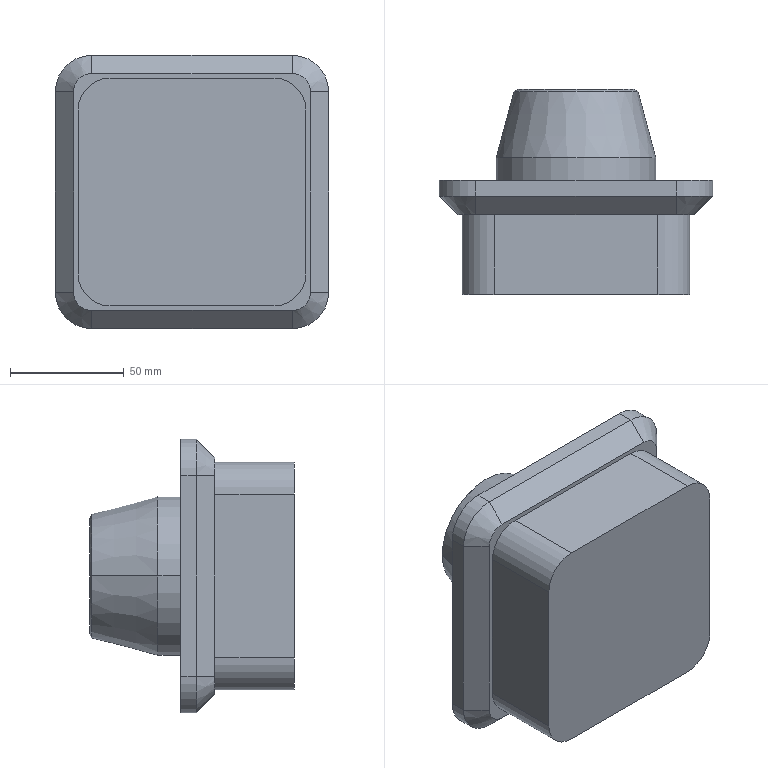Part | SolidWorks | features Chamfer 2, ICE 2, Revolution 1 | 1 solid | 34 faces | box 120 x 90 x 120 mm | volume 672208 mm3 | plane 16 | cylinder 10 | cone 8 | commonest cylinder face diameters 28 x4 32 x4 70 x2
STEP:
#1=CARTESIAN_POINT('',(-25.547,40.,0.));
#2=VERTEX_POINT('',#1);
#3=CARTESIAN_POINT('',(25.547,40.,0.));
#4=VERTEX_POINT('',#3);
#5=CARTESIAN_POINT('',(0.,40.,0.));
#6=DIRECTION('',(0.,1.,0.));
#7=DIRECTION('',(1.,0.,0.));
#8=AXIS2_PLACEMENT_3D('',#5,#6,#7);
#9=CIRCLE('',#8,25.547);
#10=EDGE_CURVE('',#2,#4,#9,.T.);
#11=ORIENTED_EDGE('',*,*,#10,.F.);
#12=CARTESIAN_POINT('',(-27.22,39.034,0.));
#13=VERTEX_POINT('',#12);
#14=CARTESIAN_POINT('',(-25.547,40.,0.));
#15=DIRECTION('',(-0.866,-0.5,0.));
#16=VECTOR('',#15,1000.);
#17=LINE('',#14,#16);
#18=EDGE_CURVE('',#2,#13,#17,.T.);
#19=ORIENTED_EDGE('',*,*,#18,.T.);
#20=CARTESIAN_POINT('',(27.22,39.034,0.));
#21=VERTEX_POINT('',#20);
#22=CARTESIAN_POINT('',(0.,39.034,0.));
#23=DIRECTION('',(0.,-1.,0.));
#24=DIRECTION('',(-1.,0.,0.));
#25=AXIS2_PLACEMENT_3D('',#22,#23,#24);
#26=CIRCLE('',#25,27.22);
#27=EDGE_CURVE('',#21,#13,#26,.T.);
#28=ORIENTED_EDGE('',*,*,#27,.F.);
#29=CARTESIAN_POINT('',(25.547,40.,0.));
#30=DIRECTION('',(0.866,-0.5,0.));
#31=VECTOR('',#30,1000.);
#32=LINE('',#29,#31);
#33=EDGE_CURVE('',#4,#21,#32,.T.);
#34=ORIENTED_EDGE('',*,*,#33,.F.);
#35=EDGE_LOOP('',(#11,#19,#28,#34));
#36=FACE_OUTER_BOUND('',#35,.T.);
#37=CARTESIAN_POINT('',(0.,40.,0.));
#38=DIRECTION('',(0.,-1.,0.));
#39=DIRECTION('',(1.,0.,0.));
#40=AXIS2_PLACEMENT_3D('',#37,#38,#39);
#41=CONICAL_SURFACE('',#40,25.547,1.047);
#42=ADVANCED_FACE('',(#36),#41,.T.);
#43=ORIENTED_EDGE('',*,*,#27,.T.);
#44=CARTESIAN_POINT('',(-35.,10.,0.));
#45=VERTEX_POINT('',#44);
#46=CARTESIAN_POINT('',(-35.,10.,0.));
#47=DIRECTION('',(-0.2588,-0.9659,0.));
#48=VECTOR('',#47,1000.);
#49=LINE('',#46,#48);
#50=EDGE_CURVE('',#13,#45,#49,.T.);
#51=ORIENTED_EDGE('',*,*,#50,.T.);
#52=CARTESIAN_POINT('',(35.,10.,0.));
#53=VERTEX_POINT('',#52);
#54=CARTESIAN_POINT('',(0.,10.,0.));
#55=DIRECTION('',(0.,1.,0.));
#56=DIRECTION('',(-1.,0.,0.));
#57=AXIS2_PLACEMENT_3D('',#54,#55,#56);
#58=CIRCLE('',#57,35.);
#59=EDGE_CURVE('',#45,#53,#58,.T.);
#60=ORIENTED_EDGE('',*,*,#59,.T.);
#61=CARTESIAN_POINT('',(35.,10.,0.));
#62=DIRECTION('',(0.2588,-0.9659,0.));
#63=VECTOR('',#62,1000.);
#64=LINE('',#61,#63);
#65=EDGE_CURVE('',#21,#53,#64,.T.);
#66=ORIENTED_EDGE('',*,*,#65,.F.);
#67=EDGE_LOOP('',(#43,#51,#60,#66));
#68=FACE_OUTER_BOUND('',#67,.T.);
#69=CARTESIAN_POINT('',(0.,10.,0.));
#70=DIRECTION('',(0.,-1.,0.));
#71=DIRECTION('',(1.,0.,0.));
#72=AXIS2_PLACEMENT_3D('',#69,#70,#71);
#73=CONICAL_SURFACE('',#72,35.,0.2618);
#74=ADVANCED_FACE('',(#68),#73,.T.);
#75=CARTESIAN_POINT('',(-35.,0.,0.));
#76=VERTEX_POINT('',#75);
#77=CARTESIAN_POINT('',(35.,0.,0.));
#78=VERTEX_POINT('',#77);
#79=CARTESIAN_POINT('',(0.,0.,0.));
#80=DIRECTION('',(0.,1.,0.));
#81=DIRECTION('',(-1.,0.,0.));
#82=AXIS2_PLACEMENT_3D('',#79,#80,#81);
#83=CIRCLE('',#82,35.);
#84=EDGE_CURVE('',#76,#78,#83,.T.);
#85=ORIENTED_EDGE('',*,*,#84,.T.);
#86=CARTESIAN_POINT('',(35.,40.,0.));
#87=DIRECTION('',(0.,1.,0.));
#88=VECTOR('',#87,1000.);
#89=LINE('',#86,#88);
#90=EDGE_CURVE('',#78,#53,#89,.T.);
#91=ORIENTED_EDGE('',*,*,#90,.T.);
#92=ORIENTED_EDGE('',*,*,#59,.F.);
#93=CARTESIAN_POINT('',(-35.,40.,0.));
#94=DIRECTION('',(0.,1.,0.));
#95=VECTOR('',#94,1000.);
#96=LINE('',#93,#95);
#97=EDGE_CURVE('',#76,#45,#96,.T.);
#98=ORIENTED_EDGE('',*,*,#97,.F.);
#99=EDGE_LOOP('',(#85,#91,#92,#98));
#100=FACE_OUTER_BOUND('',#99,.T.);
#101=CARTESIAN_POINT('',(0.,40.,0.));
#102=DIRECTION('',(0.,1.,0.));
#103=DIRECTION('',(-1.,0.,0.));
#104=AXIS2_PLACEMENT_3D('',#101,#102,#103);
#105=CYLINDRICAL_SURFACE('',#104,35.);
#106=ADVANCED_FACE('',(#100),#105,.T.);
#107=CARTESIAN_POINT('',(-52.,-15.,44.));
#108=VERTEX_POINT('',#107);
#109=CARTESIAN_POINT('',(-52.,-15.,-44.));
#110=VERTEX_POINT('',#109);
#111=CARTESIAN_POINT('',(-52.,-15.,-44.));
#112=DIRECTION('',(0.,0.,-1.));
#113=VECTOR('',#112,1000.);
#114=LINE('',#111,#113);
#115=EDGE_CURVE('',#108,#110,#114,.T.);
#116=ORIENTED_EDGE('',*,*,#115,.T.);
#117=CARTESIAN_POINT('',(-44.,-15.,-52.));
#118=VERTEX_POINT('',#117);
#119=CARTESIAN_POINT('',(-44.,-15.,-44.));
#120=DIRECTION('',(0.,-1.,0.));
#121=DIRECTION('',(-1.,0.,0.));
#122=AXIS2_PLACEMENT_3D('',#119,#120,#121);
#123=CIRCLE('',#122,8.);
#124=EDGE_CURVE('',#110,#118,#123,.T.);
#125=ORIENTED_EDGE('',*,*,#124,.T.);
#126=CARTESIAN_POINT('',(44.,-15.,-52.));
#127=VERTEX_POINT('',#126);
#128=CARTESIAN_POINT('',(-44.,-15.,-52.));
#129=DIRECTION('',(1.,0.,0.));
#130=VECTOR('',#129,1000.);
#131=LINE('',#128,#130);
#132=EDGE_CURVE('',#118,#127,#131,.T.);
#133=ORIENTED_EDGE('',*,*,#132,.T.);
#134=CARTESIAN_POINT('',(52.,-15.,-44.));
#135=VERTEX_POINT('',#134);
#136=CARTESIAN_POINT('',(44.,-15.,-44.));
#137=DIRECTION('',(0.,-1.,0.));
#138=DIRECTION('',(-1.,0.,0.));
#139=AXIS2_PLACEMENT_3D('',#136,#137,#138);
#140=CIRCLE('',#139,8.);
#141=EDGE_CURVE('',#127,#135,#140,.T.);
#142=ORIENTED_EDGE('',*,*,#141,.T.);
#143=CARTESIAN_POINT('',(52.,-15.,44.));
#144=VERTEX_POINT('',#143);
#145=CARTESIAN_POINT('',(52.,-15.,-44.));
#146=DIRECTION('',(0.,0.,1.));
#147=VECTOR('',#146,1000.);
#148=LINE('',#145,#147);
#149=EDGE_CURVE('',#135,#144,#148,.T.);
#150=ORIENTED_EDGE('',*,*,#149,.T.);
#151=CARTESIAN_POINT('',(44.,-15.,52.));
#152=VERTEX_POINT('',#151);
#153=CARTESIAN_POINT('',(44.,-15.,44.));
#154=DIRECTION('',(0.,-1.,0.));
#155=DIRECTION('',(-1.,0.,0.));
#156=AXIS2_PLACEMENT_3D('',#153,#154,#155);
#157=CIRCLE('',#156,8.);
#158=EDGE_CURVE('',#144,#152,#157,.T.);
#159=ORIENTED_EDGE('',*,*,#158,.T.);
#160=CARTESIAN_POINT('',(-44.,-15.,52.));
#161=VERTEX_POINT('',#160);
#162=CARTESIAN_POINT('',(-44.,-15.,52.));
#163=DIRECTION('',(-1.,0.,0.));
#164=VECTOR('',#163,1000.);
#165=LINE('',#162,#164);
#166=EDGE_CURVE('',#152,#161,#165,.T.);
#167=ORIENTED_EDGE('',*,*,#166,.T.);
#168=CARTESIAN_POINT('',(-44.,-15.,44.));
#169=DIRECTION('',(0.,-1.,0.));
#170=DIRECTION('',(-1.,0.,0.));
#171=AXIS2_PLACEMENT_3D('',#168,#169,#170);
#172=CIRCLE('',#171,8.);
#173=EDGE_CURVE('',#161,#108,#172,.T.);
#174=ORIENTED_EDGE('',*,*,#173,.T.);
#175=EDGE_LOOP('',(#116,#125,#133,#142,#150,#159,#167,#174));
#176=FACE_OUTER_BOUND('',#175,.T.);
#177=CARTESIAN_POINT('',(-50.,-15.,-36.));
#178=VERTEX_POINT('',#177);
#179=CARTESIAN_POINT('',(-36.,-15.,-50.));
#180=VERTEX_POINT('',#179);
#181=CARTESIAN_POINT('',(-36.,-15.,-36.));
#182=DIRECTION('',(0.,-1.,0.));
#183=DIRECTION('',(-1.,0.,0.));
#184=AXIS2_PLACEMENT_3D('',#181,#182,#183);
#185=CIRCLE('',#184,14.);
#186=EDGE_CURVE('',#178,#180,#185,.T.);
#187=ORIENTED_EDGE('',*,*,#186,.F.);
#188=CARTESIAN_POINT('',(-50.,-15.,36.));
#189=VERTEX_POINT('',#188);
#190=CARTESIAN_POINT('',(-50.,-15.,-36.));
#191=DIRECTION('',(0.,0.,-1.));
#192=VECTOR('',#191,1000.);
#193=LINE('',#190,#192);
#194=EDGE_CURVE('',#189,#178,#193,.T.);
#195=ORIENTED_EDGE('',*,*,#194,.F.);
#196=CARTESIAN_POINT('',(-36.,-15.,50.));
#197=VERTEX_POINT('',#196);
#198=CARTESIAN_POINT('',(-36.,-15.,36.));
#199=DIRECTION('',(0.,-1.,0.));
#200=DIRECTION('',(1.,0.,0.));
#201=AXIS2_PLACEMENT_3D('',#198,#199,#200);
#202=CIRCLE('',#201,14.);
#203=EDGE_CURVE('',#197,#189,#202,.T.);
#204=ORIENTED_EDGE('',*,*,#203,.F.);
#205=CARTESIAN_POINT('',(36.,-15.,50.));
#206=VERTEX_POINT('',#205);
#207=CARTESIAN_POINT('',(36.,-15.,50.));
#208=DIRECTION('',(-1.,0.,0.));
#209=VECTOR('',#208,1000.);
#210=LINE('',#207,#209);
#211=EDGE_CURVE('',#206,#197,#210,.T.);
#212=ORIENTED_EDGE('',*,*,#211,.F.);
#213=CARTESIAN_POINT('',(50.,-15.,36.));
#214=VERTEX_POINT('',#213);
#215=CARTESIAN_POINT('',(36.,-15.,36.));
#216=DIRECTION('',(0.,-1.,0.));
#217=DIRECTION('',(1.,0.,0.));
#218=AXIS2_PLACEMENT_3D('',#215,#216,#217);
#219=CIRCLE('',#218,14.);
#220=EDGE_CURVE('',#214,#206,#219,.T.);
#221=ORIENTED_EDGE('',*,*,#220,.F.);
#222=CARTESIAN_POINT('',(50.,-15.,-36.));
#223=VERTEX_POINT('',#222);
#224=CARTESIAN_POINT('',(50.,-15.,-36.));
#225=DIRECTION('',(0.,0.,1.));
#226=VECTOR('',#225,1000.);
#227=LINE('',#224,#226);
#228=EDGE_CURVE('',#223,#214,#227,.T.);
#229=ORIENTED_EDGE('',*,*,#228,.F.);
#230=CARTESIAN_POINT('',(36.,-15.,-50.));
#231=VERTEX_POINT('',#230);
#232=CARTESIAN_POINT('',(36.,-15.,-36.));
#233=DIRECTION('',(0.,-1.,0.));
#234=DIRECTION('',(1.,0.,0.));
#235=AXIS2_PLACEMENT_3D('',#232,#233,#234);
#236=CIRCLE('',#235,14.);
#237=EDGE_CURVE('',#231,#223,#236,.T.);
#238=ORIENTED_EDGE('',*,*,#237,.F.);
#239=CARTESIAN_POINT('',(36.,-15.,-50.));
#240=DIRECTION('',(1.,0.,0.));
#241=VECTOR('',#240,1000.);
#242=LINE('',#239,#241);
#243=EDGE_CURVE('',#180,#231,#242,.T.);
#244=ORIENTED_EDGE('',*,*,#243,.F.);
#245=EDGE_LOOP('',(#187,#195,#204,#212,#221,#229,#238,#244));
#246=FACE_BOUND('',#245,.T.);
#247=CARTESIAN_POINT('',(-44.,-15.,-44.));
#248=DIRECTION('',(0.,1.,0.));
#249=DIRECTION('',(-1.,0.,0.));
#250=AXIS2_PLACEMENT_3D('',#247,#248,#249);
#251=PLANE('',#250);
#252=ADVANCED_FACE('',(#176,#246),#251,.F.);
#253=ORIENTED_EDGE('',*,*,#90,.F.);
#254=CARTESIAN_POINT('',(0.,0.,0.));
#255=DIRECTION('',(0.,1.,0.));
#256=DIRECTION('',(-1.,0.,0.));
#257=AXIS2_PLACEMENT_3D('',#254,#255,#256);
#258=CIRCLE('',#257,35.);
#259=EDGE_CURVE('',#78,#76,#258,.T.);
#260=ORIENTED_EDGE('',*,*,#259,.T.);
#261=ORIENTED_EDGE('',*,*,#97,.T.);
#262=CARTESIAN_POINT('',(0.,10.,0.));
#263=DIRECTION('',(0.,1.,0.));
#264=DIRECTION('',(-1.,0.,0.));
#265=AXIS2_PLACEMENT_3D('',#262,#263,#264);
#266=CIRCLE('',#265,35.);
#267=EDGE_CURVE('',#53,#45,#266,.T.);
#268=ORIENTED_EDGE('',*,*,#267,.F.);
#269=EDGE_LOOP('',(#253,#260,#261,#268));
#270=FACE_OUTER_BOUND('',#269,.T.);
#271=CARTESIAN_POINT('',(0.,40.,0.));
#272=DIRECTION('',(0.,1.,0.));
#273=DIRECTION('',(-1.,0.,0.));
#274=AXIS2_PLACEMENT_3D('',#271,#272,#273);
#275=CYLINDRICAL_SURFACE('',#274,35.);
#276=ADVANCED_FACE('',(#270),#275,.T.);
#277=ORIENTED_EDGE('',*,*,#50,.F.);
#278=CARTESIAN_POINT('',(0.,39.034,0.));
#279=DIRECTION('',(0.,-1.,0.));
#280=DIRECTION('',(-1.,0.,0.));
#281=AXIS2_PLACEMENT_3D('',#278,#279,#280);
#282=CIRCLE('',#281,27.22);
#283=EDGE_CURVE('',#13,#21,#282,.T.);
#284=ORIENTED_EDGE('',*,*,#283,.T.);
#285=ORIENTED_EDGE('',*,*,#65,.T.);
#286=ORIENTED_EDGE('',*,*,#267,.T.);
#287=EDGE_LOOP('',(#277,#284,#285,#286));
#288=FACE_OUTER_BOUND('',#287,.T.);
#289=CARTESIAN_POINT('',(0.,10.,0.));
#290=DIRECTION('',(0.,-1.,0.));
#291=DIRECTION('',(1.,0.,0.));
#292=AXIS2_PLACEMENT_3D('',#289,#290,#291);
#293=CONICAL_SURFACE('',#292,35.,0.2618);
#294=ADVANCED_FACE('',(#288),#293,.T.);
#295=CARTESIAN_POINT('',(0.,40.,0.));
#296=DIRECTION('',(0.,1.,0.));
#297=DIRECTION('',(1.,0.,0.));
#298=AXIS2_PLACEMENT_3D('',#295,#296,#297);
#299=CIRCLE('',#298,25.547);
#300=EDGE_CURVE('',#4,#2,#299,.T.);
#301=ORIENTED_EDGE('',*,*,#300,.T.);
#302=ORIENTED_EDGE('',*,*,#10,.T.);
#303=EDGE_LOOP('',(#301,#302));
#304=FACE_OUTER_BOUND('',#303,.T.);
#305=CARTESIAN_POINT('',(26.962,40.,0.));
#306=DIRECTION('',(0.,-1.,0.));
#307=DIRECTION('',(1.,0.,0.));
#308=AXIS2_PLACEMENT_3D('',#305,#306,#307);
#309=PLANE('',#308);
#310=ADVANCED_FACE('',(#304),#309,.F.);
#311=ORIENTED_EDGE('',*,*,#18,.F.);
#312=ORIENTED_EDGE('',*,*,#300,.F.);
#313=ORIENTED_EDGE('',*,*,#33,.T.);
#314=ORIENTED_EDGE('',*,*,#283,.F.);
#315=EDGE_LOOP('',(#311,#312,#313,#314));
#316=FACE_OUTER_BOUND('',#315,.T.);
#317=CARTESIAN_POINT('',(0.,40.,0.));
#318=DIRECTION('',(0.,-1.,0.));
#319=DIRECTION('',(1.,0.,0.));
#320=AXIS2_PLACEMENT_3D('',#317,#318,#319);
#321=CONICAL_SURFACE('',#320,25.547,1.047);
#322=ADVANCED_FACE('',(#316),#321,.T.);
#323=CARTESIAN_POINT('',(-44.,-7.,-60.));
#324=VERTEX_POINT('',#323);
#325=CARTESIAN_POINT('',(-44.,0.,-60.));
#326=VERTEX_POINT('',#325);
#327=CARTESIAN_POINT('',(-44.,-15.,-60.));
#328=DIRECTION('',(0.,1.,0.));
#329=VECTOR('',#328,1000.);
#330=LINE('',#327,#329);
#331=EDGE_CURVE('',#324,#326,#330,.T.);
#332=ORIENTED_EDGE('',*,*,#331,.F.);
#333=CARTESIAN_POINT('',(-60.,-7.,-44.));
#334=VERTEX_POINT('',#333);
#335=CARTESIAN_POINT('',(-44.,-7.,-44.));
#336=DIRECTION('',(0.,1.,0.));
#337=DIRECTION('',(0.,0.,1.));
#338=AXIS2_PLACEMENT_3D('',#335,#336,#337);
#339=CIRCLE('',#338,16.);
#340=EDGE_CURVE('',#324,#334,#339,.T.);
#341=ORIENTED_EDGE('',*,*,#340,.T.);
#342=CARTESIAN_POINT('',(-60.,0.,-44.));
#343=VERTEX_POINT('',#342);
#344=CARTESIAN_POINT('',(-60.,-15.,-44.));
#345=DIRECTION('',(0.,1.,0.));
#346=VECTOR('',#345,1000.);
#347=LINE('',#344,#346);
#348=EDGE_CURVE('',#334,#343,#347,.T.);
#349=ORIENTED_EDGE('',*,*,#348,.T.);
#350=CARTESIAN_POINT('',(-44.,0.,-44.));
#351=DIRECTION('',(0.,-1.,0.));
#352=DIRECTION('',(-1.,0.,0.));
#353=AXIS2_PLACEMENT_3D('',#350,#351,#352);
#354=CIRCLE('',#353,16.);
#355=EDGE_CURVE('',#343,#326,#354,.T.);
#356=ORIENTED_EDGE('',*,*,#355,.T.);
#357=EDGE_LOOP('',(#332,#341,#349,#356));
#358=FACE_OUTER_BOUND('',#357,.T.);
#359=CARTESIAN_POINT('',(-44.,-15.,-44.));
#360=DIRECTION('',(0.,1.,0.));
#361=DIRECTION('',(-1.,0.,0.));
#362=AXIS2_PLACEMENT_3D('',#359,#360,#361);
#363=CYLINDRICAL_SURFACE('',#362,16.);
#364=ADVANCED_FACE('',(#358),#363,.T.);
#365=CARTESIAN_POINT('',(44.,-7.,-60.));
#366=VERTEX_POINT('',#365);
#367=CARTESIAN_POINT('',(44.,0.,-60.));
#368=VERTEX_POINT('',#367);
#369=CARTESIAN_POINT('',(44.,-15.,-60.));
#370=DIRECTION('',(0.,1.,0.));
#371=VECTOR('',#370,1000.);
#372=LINE('',#369,#371);
#373=EDGE_CURVE('',#366,#368,#372,.T.);
#374=ORIENTED_EDGE('',*,*,#373,.F.);
#375=CARTESIAN_POINT('',(44.,-7.,-60.));
#376=DIRECTION('',(-1.,0.,0.));
#377=VECTOR('',#376,1000.);
#378=LINE('',#375,#377);
#379=EDGE_CURVE('',#366,#324,#378,.T.);
#380=ORIENTED_EDGE('',*,*,#379,.T.);
#381=ORIENTED_EDGE('',*,*,#331,.T.);
#382=CARTESIAN_POINT('',(44.,0.,-60.));
#383=DIRECTION('',(1.,0.,0.));
#384=VECTOR('',#383,1000.);
#385=LINE('',#382,#384);
#386=EDGE_CURVE('',#326,#368,#385,.T.);
#387=ORIENTED_EDGE('',*,*,#386,.T.);
#388=EDGE_LOOP('',(#374,#380,#381,#387));
#389=FACE_OUTER_BOUND('',#388,.T.);
#390=CARTESIAN_POINT('',(44.,-15.,-60.));
#391=DIRECTION('',(0.,0.,1.));
#392=DIRECTION('',(1.,0.,0.));
#393=AXIS2_PLACEMENT_3D('',#390,#391,#392);
#394=PLANE('',#393);
#395=ADVANCED_FACE('',(#389),#394,.F.);
#396=CARTESIAN_POINT('',(60.,-7.,-44.));
#397=VERTEX_POINT('',#396);
#398=CARTESIAN_POINT('',(60.,0.,-44.));
#399=VERTEX_POINT('',#398);
#400=CARTESIAN_POINT('',(60.,-15.,-44.));
#401=DIRECTION('',(0.,1.,0.));
#402=VECTOR('',#401,1000.);
#403=LINE('',#400,#402);
#404=EDGE_CURVE('',#397,#399,#403,.T.);
#405=ORIENTED_EDGE('',*,*,#404,.F.);
#406=CARTESIAN_POINT('',(44.,-7.,-44.));
#407=DIRECTION('',(0.,1.,0.));
#408=DIRECTION('',(0.,0.,1.));
#409=AXIS2_PLACEMENT_3D('',#406,#407,#408);
#410=CIRCLE('',#409,16.);
#411=EDGE_CURVE('',#397,#366,#410,.T.);
#412=ORIENTED_EDGE('',*,*,#411,.T.);
#413=ORIENTED_EDGE('',*,*,#373,.T.);
#414=CARTESIAN_POINT('',(44.,0.,-44.));
#415=DIRECTION('',(0.,-1.,0.));
#416=DIRECTION('',(1.,0.,0.));
#417=AXIS2_PLACEMENT_3D('',#414,#415,#416);
#418=CIRCLE('',#417,16.);
#419=EDGE_CURVE('',#368,#399,#418,.T.);
#420=ORIENTED_EDGE('',*,*,#419,.T.);
#421=EDGE_LOOP('',(#405,#412,#413,#420));
#422=FACE_OUTER_BOUND('',#421,.T.);
#423=CARTESIAN_POINT('',(44.,-15.,-44.));
#424=DIRECTION('',(0.,1.,0.));
#425=DIRECTION('',(-1.,0.,0.));
#426=AXIS2_PLACEMENT_3D('',#423,#424,#425);
#427=CYLINDRICAL_SURFACE('',#426,16.);
#428=ADVANCED_FACE('',(#422),#427,.T.);
#429=CARTESIAN_POINT('',(60.,-7.,44.));
#430=VERTEX_POINT('',#429);
#431=CARTESIAN_POINT('',(60.,0.,44.));
#432=VERTEX_POINT('',#431);
#433=CARTESIAN_POINT('',(60.,-15.,44.));
#434=DIRECTION('',(0.,1.,0.));
#435=VECTOR('',#434,1000.);
#436=LINE('',#433,#435);
#437=EDGE_CURVE('',#430,#432,#436,.T.);
#438=ORIENTED_EDGE('',*,*,#437,.F.);
#439=CARTESIAN_POINT('',(60.,-7.,-44.));
#440=DIRECTION('',(0.,0.,-1.));
#441=VECTOR('',#440,1000.);
#442=LINE('',#439,#441);
#443=EDGE_CURVE('',#430,#397,#442,.T.);
#444=ORIENTED_EDGE('',*,*,#443,.T.);
#445=ORIENTED_EDGE('',*,*,#404,.T.);
#446=CARTESIAN_POINT('',(60.,0.,-44.));
#447=DIRECTION('',(0.,0.,1.));
#448=VECTOR('',#447,1000.);
#449=LINE('',#446,#448);
#450=EDGE_CURVE('',#399,#432,#449,.T.);
#451=ORIENTED_EDGE('',*,*,#450,.T.);
#452=EDGE_LOOP('',(#438,#444,#445,#451));
#453=FACE_OUTER_BOUND('',#452,.T.);
#454=CARTESIAN_POINT('',(60.,-15.,-44.));
#455=DIRECTION('',(-1.,0.,0.));
#456=DIRECTION('',(0.,-1.,0.));
#457=AXIS2_PLACEMENT_3D('',#454,#455,#456);
#458=PLANE('',#457);
#459=ADVANCED_FACE('',(#453),#458,.F.);
#460=CARTESIAN_POINT('',(44.,-7.,60.));
#461=VERTEX_POINT('',#460);
#462=CARTESIAN_POINT('',(44.,0.,60.));
#463=VERTEX_POINT('',#462);
#464=CARTESIAN_POINT('',(44.,-15.,60.));
#465=DIRECTION('',(0.,1.,0.));
#466=VECTOR('',#465,1000.);
#467=LINE('',#464,#466);
#468=EDGE_CURVE('',#461,#463,#467,.T.);
#469=ORIENTED_EDGE('',*,*,#468,.F.);
#470=CARTESIAN_POINT('',(44.,-7.,44.));
#471=DIRECTION('',(0.,1.,0.));
#472=DIRECTION('',(0.,0.,1.));
#473=AXIS2_PLACEMENT_3D('',#470,#471,#472);
#474=CIRCLE('',#473,16.);
#475=EDGE_CURVE('',#461,#430,#474,.T.);
#476=ORIENTED_EDGE('',*,*,#475,.T.);
#477=ORIENTED_EDGE('',*,*,#437,.T.);
#478=CARTESIAN_POINT('',(44.,0.,44.));
#479=DIRECTION('',(0.,-1.,0.));
#480=DIRECTION('',(1.,0.,0.));
#481=AXIS2_PLACEMENT_3D('',#478,#479,#480);
#482=CIRCLE('',#481,16.);
#483=EDGE_CURVE('',#432,#463,#482,.T.);
#484=ORIENTED_EDGE('',*,*,#483,.T.);
#485=EDGE_LOOP('',(#469,#476,#477,#484));
#486=FACE_OUTER_BOUND('',#485,.T.);
#487=CARTESIAN_POINT('',(44.,-15.,44.));
#488=DIRECTION('',(0.,1.,0.));
#489=DIRECTION('',(-1.,0.,0.));
#490=AXIS2_PLACEMENT_3D('',#487,#488,#489);
#491=CYLINDRICAL_SURFACE('',#490,16.);
#492=ADVANCED_FACE('',(#486),#491,.T.);
#493=CARTESIAN_POINT('',(-44.,-7.,60.));
#494=VERTEX_POINT('',#493);
#495=CARTESIAN_POINT('',(-44.,0.,60.));
#496=VERTEX_POINT('',#495);
#497=CARTESIAN_POINT('',(-44.,-15.,60.));
#498=DIRECTION('',(0.,1.,0.));
#499=VECTOR('',#498,1000.);
#500=LINE('',#497,#499);
#501=EDGE_CURVE('',#494,#496,#500,.T.);
#502=ORIENTED_EDGE('',*,*,#501,.F.);
#503=CARTESIAN_POINT('',(44.,-7.,60.));
#504=DIRECTION('',(1.,0.,0.));
#505=VECTOR('',#504,1000.);
#506=LINE('',#503,#505);
#507=EDGE_CURVE('',#494,#461,#506,.T.);
#508=ORIENTED_EDGE('',*,*,#507,.T.);
#509=ORIENTED_EDGE('',*,*,#468,.T.);
#510=CARTESIAN_POINT('',(44.,0.,60.));
#511=DIRECTION('',(-1.,0.,0.));
#512=VECTOR('',#511,1000.);
#513=LINE('',#510,#512);
#514=EDGE_CURVE('',#463,#496,#513,.T.);
#515=ORIENTED_EDGE('',*,*,#514,.T.);
#516=EDGE_LOOP('',(#502,#508,#509,#515));
#517=FACE_OUTER_BOUND('',#516,.T.);
#518=CARTESIAN_POINT('',(44.,-15.,60.));
#519=DIRECTION('',(0.,0.,-1.));
#520=DIRECTION('',(-1.,0.,0.));
#521=AXIS2_PLACEMENT_3D('',#518,#519,#520);
#522=PLANE('',#521);
#523=ADVANCED_FACE('',(#517),#522,.F.);
#524=CARTESIAN_POINT('',(-60.,-7.,44.));
#525=VERTEX_POINT('',#524);
#526=CARTESIAN_POINT('',(-60.,0.,44.));
#527=VERTEX_POINT('',#526);
#528=CARTESIAN_POINT('',(-60.,-15.,44.));
#529=DIRECTION('',(0.,1.,0.));
#530=VECTOR('',#529,1000.);
#531=LINE('',#528,#530);
#532=EDGE_CURVE('',#525,#527,#531,.T.);
#533=ORIENTED_EDGE('',*,*,#532,.F.);
#534=CARTESIAN_POINT('',(-44.,-7.,44.));
#535=DIRECTION('',(0.,1.,0.));
#536=DIRECTION('',(0.,0.,1.));
#537=AXIS2_PLACEMENT_3D('',#534,#535,#536);
#538=CIRCLE('',#537,16.);
#539=EDGE_CURVE('',#525,#494,#538,.T.);
#540=ORIENTED_EDGE('',*,*,#539,.T.);
#541=ORIENTED_EDGE('',*,*,#501,.T.);
#542=CARTESIAN_POINT('',(-44.,0.,44.));
#543=DIRECTION('',(0.,-1.,0.));
#544=DIRECTION('',(1.,0.,0.));
#545=AXIS2_PLACEMENT_3D('',#542,#543,#544);
#546=CIRCLE('',#545,16.);
#547=EDGE_CURVE('',#496,#527,#546,.T.);
#548=ORIENTED_EDGE('',*,*,#547,.T.);
#549=EDGE_LOOP('',(#533,#540,#541,#548));
#550=FACE_OUTER_BOUND('',#549,.T.);
#551=CARTESIAN_POINT('',(-44.,-15.,44.));
#552=DIRECTION('',(0.,1.,0.));
#553=DIRECTION('',(-1.,0.,0.));
#554=AXIS2_PLACEMENT_3D('',#551,#552,#553);
#555=CYLINDRICAL_SURFACE('',#554,16.);
#556=ADVANCED_FACE('',(#550),#555,.T.);
#557=ORIENTED_EDGE('',*,*,#348,.F.);
#558=CARTESIAN_POINT('',(-60.,-7.,-44.));
#559=DIRECTION('',(0.,0.,1.));
#560=VECTOR('',#559,1000.);
#561=LINE('',#558,#560);
#562=EDGE_CURVE('',#334,#525,#561,.T.);
#563=ORIENTED_EDGE('',*,*,#562,.T.);
#564=ORIENTED_EDGE('',*,*,#532,.T.);
#565=CARTESIAN_POINT('',(-60.,0.,-44.));
#566=DIRECTION('',(0.,0.,-1.));
#567=VECTOR('',#566,1000.);
#568=LINE('',#565,#567);
#569=EDGE_CURVE('',#527,#343,#568,.T.);
#570=ORIENTED_EDGE('',*,*,#569,.T.);
#571=EDGE_LOOP('',(#557,#563,#564,#570));
#572=FACE_OUTER_BOUND('',#571,.T.);
#573=CARTESIAN_POINT('',(-60.,-15.,-44.));
#574=DIRECTION('',(1.,0.,0.));
#575=DIRECTION('',(0.,0.,-1.));
#576=AXIS2_PLACEMENT_3D('',#573,#574,#575);
#577=PLANE('',#576);
#578=ADVANCED_FACE('',(#572),#577,.F.);
#579=ORIENTED_EDGE('',*,*,#84,.F.);
#580=ORIENTED_EDGE('',*,*,#259,.F.);
#581=EDGE_LOOP('',(#579,#580));
#582=FACE_BOUND('',#581,.T.);
#583=ORIENTED_EDGE('',*,*,#355,.F.);
#584=ORIENTED_EDGE('',*,*,#569,.F.);
#585=ORIENTED_EDGE('',*,*,#547,.F.);
#586=ORIENTED_EDGE('',*,*,#514,.F.);
#587=ORIENTED_EDGE('',*,*,#483,.F.);
#588=ORIENTED_EDGE('',*,*,#450,.F.);
#589=ORIENTED_EDGE('',*,*,#419,.F.);
#590=ORIENTED_EDGE('',*,*,#386,.F.);
#591=EDGE_LOOP('',(#583,#584,#585,#586,#587,#588,#589,#590));
#592=FACE_OUTER_BOUND('',#591,.T.);
#593=CARTESIAN_POINT('',(-44.,0.,-44.));
#594=DIRECTION('',(0.,1.,0.));
#595=DIRECTION('',(-1.,0.,0.));
#596=AXIS2_PLACEMENT_3D('',#593,#594,#595);
#597=PLANE('',#596);
#598=ADVANCED_FACE('',(#582,#592),#597,.T.);
#599=ORIENTED_EDGE('',*,*,#186,.T.);
#600=CARTESIAN_POINT('',(-36.,-50.,-50.));
#601=VERTEX_POINT('',#600);
#602=CARTESIAN_POINT('',(-36.,-50.,-50.));
#603=DIRECTION('',(0.,1.,0.));
#604=VECTOR('',#603,1000.);
#605=LINE('',#602,#604);
#606=EDGE_CURVE('',#601,#180,#605,.T.);
#607=ORIENTED_EDGE('',*,*,#606,.F.);
#608=CARTESIAN_POINT('',(-50.,-50.,-36.));
#609=VERTEX_POINT('',#608);
#610=CARTESIAN_POINT('',(-36.,-50.,-36.));
#611=DIRECTION('',(0.,-1.,0.));
#612=DIRECTION('',(-1.,0.,0.));
#613=AXIS2_PLACEMENT_3D('',#610,#611,#612);
#614=CIRCLE('',#613,14.);
#615=EDGE_CURVE('',#609,#601,#614,.T.);
#616=ORIENTED_EDGE('',*,*,#615,.F.);
#617=CARTESIAN_POINT('',(-50.,-50.,-36.));
#618=DIRECTION('',(0.,1.,0.));
#619=VECTOR('',#618,1000.);
#620=LINE('',#617,#619);
#621=EDGE_CURVE('',#609,#178,#620,.T.);
#622=ORIENTED_EDGE('',*,*,#621,.T.);
#623=EDGE_LOOP('',(#599,#607,#616,#622));
#624=FACE_OUTER_BOUND('',#623,.T.);
#625=CARTESIAN_POINT('',(-36.,-50.,-36.));
#626=DIRECTION('',(0.,1.,0.));
#627=DIRECTION('',(-1.,0.,0.));
#628=AXIS2_PLACEMENT_3D('',#625,#626,#627);
#629=CYLINDRICAL_SURFACE('',#628,14.);
#630=ADVANCED_FACE('',(#624),#629,.T.);
#631=ORIENTED_EDGE('',*,*,#243,.T.);
#632=CARTESIAN_POINT('',(36.,-50.,-50.));
#633=VERTEX_POINT('',#632);
#634=CARTESIAN_POINT('',(36.,-50.,-50.));
#635=DIRECTION('',(0.,1.,0.));
#636=VECTOR('',#635,1000.);
#637=LINE('',#634,#636);
#638=EDGE_CURVE('',#633,#231,#637,.T.);
#639=ORIENTED_EDGE('',*,*,#638,.F.);
#640=CARTESIAN_POINT('',(36.,-50.,-50.));
#641=DIRECTION('',(1.,0.,0.));
#642=VECTOR('',#641,1000.);
#643=LINE('',#640,#642);
#644=EDGE_CURVE('',#601,#633,#643,.T.);
#645=ORIENTED_EDGE('',*,*,#644,.F.);
#646=ORIENTED_EDGE('',*,*,#606,.T.);
#647=EDGE_LOOP('',(#631,#639,#645,#646));
#648=FACE_OUTER_BOUND('',#647,.T.);
#649=CARTESIAN_POINT('',(36.,-50.,-50.));
#650=DIRECTION('',(0.,0.,1.));
#651=DIRECTION('',(1.,0.,0.));
#652=AXIS2_PLACEMENT_3D('',#649,#650,#651);
#653=PLANE('',#652);
#654=ADVANCED_FACE('',(#648),#653,.F.);
#655=ORIENTED_EDGE('',*,*,#237,.T.);
#656=CARTESIAN_POINT('',(50.,-50.,-36.));
#657=VERTEX_POINT('',#656);
#658=CARTESIAN_POINT('',(50.,-50.,-36.));
#659=DIRECTION('',(0.,1.,0.));
#660=VECTOR('',#659,1000.);
#661=LINE('',#658,#660);
#662=EDGE_CURVE('',#657,#223,#661,.T.);
#663=ORIENTED_EDGE('',*,*,#662,.F.);
#664=CARTESIAN_POINT('',(36.,-50.,-36.));
#665=DIRECTION('',(0.,-1.,0.));
#666=DIRECTION('',(1.,0.,0.));
#667=AXIS2_PLACEMENT_3D('',#664,#665,#666);
#668=CIRCLE('',#667,14.);
#669=EDGE_CURVE('',#633,#657,#668,.T.);
#670=ORIENTED_EDGE('',*,*,#669,.F.);
#671=ORIENTED_EDGE('',*,*,#638,.T.);
#672=EDGE_LOOP('',(#655,#663,#670,#671));
#673=FACE_OUTER_BOUND('',#672,.T.);
#674=CARTESIAN_POINT('',(36.,-50.,-36.));
#675=DIRECTION('',(0.,1.,0.));
#676=DIRECTION('',(-1.,0.,0.));
#677=AXIS2_PLACEMENT_3D('',#674,#675,#676);
#678=CYLINDRICAL_SURFACE('',#677,14.);
#679=ADVANCED_FACE('',(#673),#678,.T.);
#680=ORIENTED_EDGE('',*,*,#228,.T.);
#681=CARTESIAN_POINT('',(50.,-50.,36.));
#682=VERTEX_POINT('',#681);
#683=CARTESIAN_POINT('',(50.,-50.,36.));
#684=DIRECTION('',(0.,1.,0.));
#685=VECTOR('',#684,1000.);
#686=LINE('',#683,#685);
#687=EDGE_CURVE('',#682,#214,#686,.T.);
#688=ORIENTED_EDGE('',*,*,#687,.F.);
#689=CARTESIAN_POINT('',(50.,-50.,-36.));
#690=DIRECTION('',(0.,0.,1.));
#691=VECTOR('',#690,1000.);
#692=LINE('',#689,#691);
#693=EDGE_CURVE('',#657,#682,#692,.T.);
#694=ORIENTED_EDGE('',*,*,#693,.F.);
#695=ORIENTED_EDGE('',*,*,#662,.T.);
#696=EDGE_LOOP('',(#680,#688,#694,#695));
#697=FACE_OUTER_BOUND('',#696,.T.);
#698=CARTESIAN_POINT('',(50.,-50.,-36.));
#699=DIRECTION('',(-1.,0.,0.));
#700=DIRECTION('',(0.,0.,1.));
#701=AXIS2_PLACEMENT_3D('',#698,#699,#700);
#702=PLANE('',#701);
#703=ADVANCED_FACE('',(#697),#702,.F.);
#704=ORIENTED_EDGE('',*,*,#220,.T.);
#705=CARTESIAN_POINT('',(36.,-50.,50.));
#706=VERTEX_POINT('',#705);
#707=CARTESIAN_POINT('',(36.,-50.,50.));
#708=DIRECTION('',(0.,1.,0.));
#709=VECTOR('',#708,1000.);
#710=LINE('',#707,#709);
#711=EDGE_CURVE('',#706,#206,#710,.T.);
#712=ORIENTED_EDGE('',*,*,#711,.F.);
#713=CARTESIAN_POINT('',(36.,-50.,36.));
#714=DIRECTION('',(0.,-1.,0.));
#715=DIRECTION('',(1.,0.,0.));
#716=AXIS2_PLACEMENT_3D('',#713,#714,#715);
#717=CIRCLE('',#716,14.);
#718=EDGE_CURVE('',#682,#706,#717,.T.);
#719=ORIENTED_EDGE('',*,*,#718,.F.);
#720=ORIENTED_EDGE('',*,*,#687,.T.);
#721=EDGE_LOOP('',(#704,#712,#719,#720));
#722=FACE_OUTER_BOUND('',#721,.T.);
#723=CARTESIAN_POINT('',(36.,-50.,36.));
#724=DIRECTION('',(0.,1.,0.));
#725=DIRECTION('',(-1.,0.,0.));
#726=AXIS2_PLACEMENT_3D('',#723,#724,#725);
#727=CYLINDRICAL_SURFACE('',#726,14.);
#728=ADVANCED_FACE('',(#722),#727,.T.);
#729=ORIENTED_EDGE('',*,*,#211,.T.);
#730=CARTESIAN_POINT('',(-36.,-50.,50.));
#731=VERTEX_POINT('',#730);
#732=CARTESIAN_POINT('',(-36.,-50.,50.));
#733=DIRECTION('',(0.,1.,0.));
#734=VECTOR('',#733,1000.);
#735=LINE('',#732,#734);
#736=EDGE_CURVE('',#731,#197,#735,.T.);
#737=ORIENTED_EDGE('',*,*,#736,.F.);
#738=CARTESIAN_POINT('',(36.,-50.,50.));
#739=DIRECTION('',(-1.,0.,0.));
#740=VECTOR('',#739,1000.);
#741=LINE('',#738,#740);
#742=EDGE_CURVE('',#706,#731,#741,.T.);
#743=ORIENTED_EDGE('',*,*,#742,.F.);
#744=ORIENTED_EDGE('',*,*,#711,.T.);
#745=EDGE_LOOP('',(#729,#737,#743,#744));
#746=FACE_OUTER_BOUND('',#745,.T.);
#747=CARTESIAN_POINT('',(36.,-50.,50.));
#748=DIRECTION('',(0.,0.,-1.));
#749=DIRECTION('',(-1.,0.,0.));
#750=AXIS2_PLACEMENT_3D('',#747,#748,#749);
#751=PLANE('',#750);
#752=ADVANCED_FACE('',(#746),#751,.F.);
#753=ORIENTED_EDGE('',*,*,#203,.T.);
#754=CARTESIAN_POINT('',(-50.,-50.,36.));
#755=VERTEX_POINT('',#754);
#756=CARTESIAN_POINT('',(-50.,-50.,36.));
#757=DIRECTION('',(0.,1.,0.));
#758=VECTOR('',#757,1000.);
#759=LINE('',#756,#758);
#760=EDGE_CURVE('',#755,#189,#759,.T.);
#761=ORIENTED_EDGE('',*,*,#760,.F.);
#762=CARTESIAN_POINT('',(-36.,-50.,36.));
#763=DIRECTION('',(0.,-1.,0.));
#764=DIRECTION('',(1.,0.,0.));
#765=AXIS2_PLACEMENT_3D('',#762,#763,#764);
#766=CIRCLE('',#765,14.);
#767=EDGE_CURVE('',#731,#755,#766,.T.);
#768=ORIENTED_EDGE('',*,*,#767,.F.);
#769=ORIENTED_EDGE('',*,*,#736,.T.);
#770=EDGE_LOOP('',(#753,#761,#768,#769));
#771=FACE_OUTER_BOUND('',#770,.T.);
#772=CARTESIAN_POINT('',(-36.,-50.,36.));
#773=DIRECTION('',(0.,1.,0.));
#774=DIRECTION('',(-1.,0.,0.));
#775=AXIS2_PLACEMENT_3D('',#772,#773,#774);
#776=CYLINDRICAL_SURFACE('',#775,14.);
#777=ADVANCED_FACE('',(#771),#776,.T.);
#778=ORIENTED_EDGE('',*,*,#194,.T.);
#779=ORIENTED_EDGE('',*,*,#621,.F.);
#780=CARTESIAN_POINT('',(-50.,-50.,-36.));
#781=DIRECTION('',(0.,0.,-1.));
#782=VECTOR('',#781,1000.);
#783=LINE('',#780,#782);
#784=EDGE_CURVE('',#755,#609,#783,.T.);
#785=ORIENTED_EDGE('',*,*,#784,.F.);
#786=ORIENTED_EDGE('',*,*,#760,.T.);
#787=EDGE_LOOP('',(#778,#779,#785,#786));
#788=FACE_OUTER_BOUND('',#787,.T.);
#789=CARTESIAN_POINT('',(-50.,-50.,-36.));
#790=DIRECTION('',(1.,0.,0.));
#791=DIRECTION('',(0.,1.,0.));
#792=AXIS2_PLACEMENT_3D('',#789,#790,#791);
#793=PLANE('',#792);
#794=ADVANCED_FACE('',(#788),#793,.F.);
#795=ORIENTED_EDGE('',*,*,#615,.T.);
#796=ORIENTED_EDGE('',*,*,#644,.T.);
#797=ORIENTED_EDGE('',*,*,#669,.T.);
#798=ORIENTED_EDGE('',*,*,#693,.T.);
#799=ORIENTED_EDGE('',*,*,#718,.T.);
#800=ORIENTED_EDGE('',*,*,#742,.T.);
#801=ORIENTED_EDGE('',*,*,#767,.T.);
#802=ORIENTED_EDGE('',*,*,#784,.T.);
#803=EDGE_LOOP('',(#795,#796,#797,#798,#799,#800,#801,#802));
#804=FACE_OUTER_BOUND('',#803,.T.);
#805=CARTESIAN_POINT('',(-36.,-50.,-36.));
#806=DIRECTION('',(0.,1.,0.));
#807=DIRECTION('',(-1.,0.,0.));
#808=AXIS2_PLACEMENT_3D('',#805,#806,#807);
#809=PLANE('',#808);
#810=ADVANCED_FACE('',(#804),#809,.F.);
#811=CARTESIAN_POINT('',(60.,-7.,44.));
#812=DIRECTION('',(-0.7071,-0.7071,0.));
#813=VECTOR('',#812,1000.);
#814=LINE('',#811,#813);
#815=EDGE_CURVE('',#430,#144,#814,.T.);
#816=ORIENTED_EDGE('',*,*,#815,.F.);
#817=ORIENTED_EDGE('',*,*,#475,.F.);
#818=CARTESIAN_POINT('',(44.,-15.,52.));
#819=DIRECTION('',(0.,0.7071,0.7071));
#820=VECTOR('',#819,1000.);
#821=LINE('',#818,#820);
#822=EDGE_CURVE('',#152,#461,#821,.T.);
#823=ORIENTED_EDGE('',*,*,#822,.F.);
#824=ORIENTED_EDGE('',*,*,#158,.F.);
#825=EDGE_LOOP('',(#816,#817,#823,#824));
#826=FACE_OUTER_BOUND('',#825,.T.);
#827=CARTESIAN_POINT('',(44.,-15.,44.));
#828=DIRECTION('',(0.,1.,0.));
#829=DIRECTION('',(0.,0.,1.));
#830=AXIS2_PLACEMENT_3D('',#827,#828,#829);
#831=CONICAL_SURFACE('',#830,8.,0.7854);
#832=ADVANCED_FACE('',(#826),#831,.T.);
#833=ORIENTED_EDGE('',*,*,#822,.T.);
#834=ORIENTED_EDGE('',*,*,#507,.F.);
#835=CARTESIAN_POINT('',(-44.,-15.,52.));
#836=DIRECTION('',(0.,0.7071,0.7071));
#837=VECTOR('',#836,1000.);
#838=LINE('',#835,#837);
#839=EDGE_CURVE('',#161,#494,#838,.T.);
#840=ORIENTED_EDGE('',*,*,#839,.F.);
#841=ORIENTED_EDGE('',*,*,#166,.F.);
#842=EDGE_LOOP('',(#833,#834,#840,#841));
#843=FACE_OUTER_BOUND('',#842,.T.);
#844=CARTESIAN_POINT('',(-44.,-15.,52.));
#845=DIRECTION('',(0.,0.7071,-0.7071));
#846=DIRECTION('',(-1.,0.,0.));
#847=AXIS2_PLACEMENT_3D('',#844,#845,#846);
#848=PLANE('',#847);
#849=ADVANCED_FACE('',(#843),#848,.F.);
#850=ORIENTED_EDGE('',*,*,#815,.T.);
#851=ORIENTED_EDGE('',*,*,#149,.F.);
#852=CARTESIAN_POINT('',(60.,-7.,-44.));
#853=DIRECTION('',(-0.7071,-0.7071,0.));
#854=VECTOR('',#853,1000.);
#855=LINE('',#852,#854);
#856=EDGE_CURVE('',#397,#135,#855,.T.);
#857=ORIENTED_EDGE('',*,*,#856,.F.);
#858=ORIENTED_EDGE('',*,*,#443,.F.);
#859=EDGE_LOOP('',(#850,#851,#857,#858));
#860=FACE_OUTER_BOUND('',#859,.T.);
#861=CARTESIAN_POINT('',(52.,-15.,-44.));
#862=DIRECTION('',(-0.7071,0.7071,0.));
#863=DIRECTION('',(0.,0.,1.));
#864=AXIS2_PLACEMENT_3D('',#861,#862,#863);
#865=PLANE('',#864);
#866=ADVANCED_FACE('',(#860),#865,.F.);
#867=ORIENTED_EDGE('',*,*,#839,.T.);
#868=ORIENTED_EDGE('',*,*,#539,.F.);
#869=CARTESIAN_POINT('',(-52.,-15.,44.));
#870=DIRECTION('',(-0.7071,0.7071,0.));
#871=VECTOR('',#870,1000.);
#872=LINE('',#869,#871);
#873=EDGE_CURVE('',#108,#525,#872,.T.);
#874=ORIENTED_EDGE('',*,*,#873,.F.);
#875=ORIENTED_EDGE('',*,*,#173,.F.);
#876=EDGE_LOOP('',(#867,#868,#874,#875));
#877=FACE_OUTER_BOUND('',#876,.T.);
#878=CARTESIAN_POINT('',(-44.,-15.,44.));
#879=DIRECTION('',(0.,1.,0.));
#880=DIRECTION('',(0.,0.,1.));
#881=AXIS2_PLACEMENT_3D('',#878,#879,#880);
#882=CONICAL_SURFACE('',#881,8.,0.7854);
#883=ADVANCED_FACE('',(#877),#882,.T.);
#884=ORIENTED_EDGE('',*,*,#856,.T.);
#885=ORIENTED_EDGE('',*,*,#141,.F.);
#886=CARTESIAN_POINT('',(44.,-7.,-60.));
#887=DIRECTION('',(0.,-0.7071,0.7071));
#888=VECTOR('',#887,1000.);
#889=LINE('',#886,#888);
#890=EDGE_CURVE('',#366,#127,#889,.T.);
#891=ORIENTED_EDGE('',*,*,#890,.F.);
#892=ORIENTED_EDGE('',*,*,#411,.F.);
#893=EDGE_LOOP('',(#884,#885,#891,#892));
#894=FACE_OUTER_BOUND('',#893,.T.);
#895=CARTESIAN_POINT('',(44.,-15.,-44.));
#896=DIRECTION('',(0.,1.,0.));
#897=DIRECTION('',(0.,0.,1.));
#898=AXIS2_PLACEMENT_3D('',#895,#896,#897);
#899=CONICAL_SURFACE('',#898,8.,0.7854);
#900=ADVANCED_FACE('',(#894),#899,.T.);
#901=ORIENTED_EDGE('',*,*,#873,.T.);
#902=ORIENTED_EDGE('',*,*,#562,.F.);
#903=CARTESIAN_POINT('',(-52.,-15.,-44.));
#904=DIRECTION('',(-0.7071,0.7071,0.));
#905=VECTOR('',#904,1000.);
#906=LINE('',#903,#905);
#907=EDGE_CURVE('',#110,#334,#906,.T.);
#908=ORIENTED_EDGE('',*,*,#907,.F.);
#909=ORIENTED_EDGE('',*,*,#115,.F.);
#910=EDGE_LOOP('',(#901,#902,#908,#909));
#911=FACE_OUTER_BOUND('',#910,.T.);
#912=CARTESIAN_POINT('',(-52.,-15.,-44.));
#913=DIRECTION('',(0.7071,0.7071,0.));
#914=DIRECTION('',(0.,0.,-1.));
#915=AXIS2_PLACEMENT_3D('',#912,#913,#914);
#916=PLANE('',#915);
#917=ADVANCED_FACE('',(#911),#916,.F.);
#918=ORIENTED_EDGE('',*,*,#890,.T.);
#919=ORIENTED_EDGE('',*,*,#132,.F.);
#920=CARTESIAN_POINT('',(-44.,-7.,-60.));
#921=DIRECTION('',(0.,-0.7071,0.7071));
#922=VECTOR('',#921,1000.);
#923=LINE('',#920,#922);
#924=EDGE_CURVE('',#324,#118,#923,.T.);
#925=ORIENTED_EDGE('',*,*,#924,.F.);
#926=ORIENTED_EDGE('',*,*,#379,.F.);
#927=EDGE_LOOP('',(#918,#919,#925,#926));
#928=FACE_OUTER_BOUND('',#927,.T.);
#929=CARTESIAN_POINT('',(-44.,-15.,-52.));
#930=DIRECTION('',(0.,0.7071,0.7071));
#931=DIRECTION('',(1.,0.,0.));
#932=AXIS2_PLACEMENT_3D('',#929,#930,#931);
#933=PLANE('',#932);
#934=ADVANCED_FACE('',(#928),#933,.F.);
#935=ORIENTED_EDGE('',*,*,#907,.T.);
#936=ORIENTED_EDGE('',*,*,#340,.F.);
#937=ORIENTED_EDGE('',*,*,#924,.T.);
#938=ORIENTED_EDGE('',*,*,#124,.F.);
#939=EDGE_LOOP('',(#935,#936,#937,#938));
#940=FACE_OUTER_BOUND('',#939,.T.);
#941=CARTESIAN_POINT('',(-44.,-15.,-44.));
#942=DIRECTION('',(0.,1.,0.));
#943=DIRECTION('',(0.,0.,1.));
#944=AXIS2_PLACEMENT_3D('',#941,#942,#943);
#945=CONICAL_SURFACE('',#944,8.,0.7854);
#946=ADVANCED_FACE('',(#940),#945,.T.);
#947=CLOSED_SHELL('',(#42,#74,#106,#252,#276,#294,#310,#322,#364,#395,#428,#459,#492,#523,#556,#578,#598,#630,#654,#679,#703,#728,#752,#777,#794,#810,#832,#849,#866,#883,#900,#917,#934,#946));
#948=MANIFOLD_SOLID_BREP('',#947);
#949=CARTESIAN_POINT('',(0.,0.,0.));
#950=DIRECTION('',(0.,0.,1.));
#951=DIRECTION('',(1.,0.,0.));
#952=AXIS2_PLACEMENT_3D('',#949,#950,#951);
#953=(LENGTH_UNIT()NAMED_UNIT(*)SI_UNIT(.MILLI.,.METRE.));
#954=UNCERTAINTY_MEASURE_WITH_UNIT(LENGTH_MEASURE(0.00001),#953,'','');
#955=(NAMED_UNIT(*)PLANE_ANGLE_UNIT()SI_UNIT($,.RADIAN.));
#956=(NAMED_UNIT(*)SI_UNIT($,.STERADIAN.)SOLID_ANGLE_UNIT());
#957=(GEOMETRIC_REPRESENTATION_CONTEXT(3)GLOBAL_UNCERTAINTY_ASSIGNED_CONTEXT((#954))GLOBAL_UNIT_ASSIGNED_CONTEXT((#953,#955,#956))REPRESENTATION_CONTEXT('',''));
#958=ADVANCED_BREP_SHAPE_REPRESENTATION('',(#948,#952),#957);